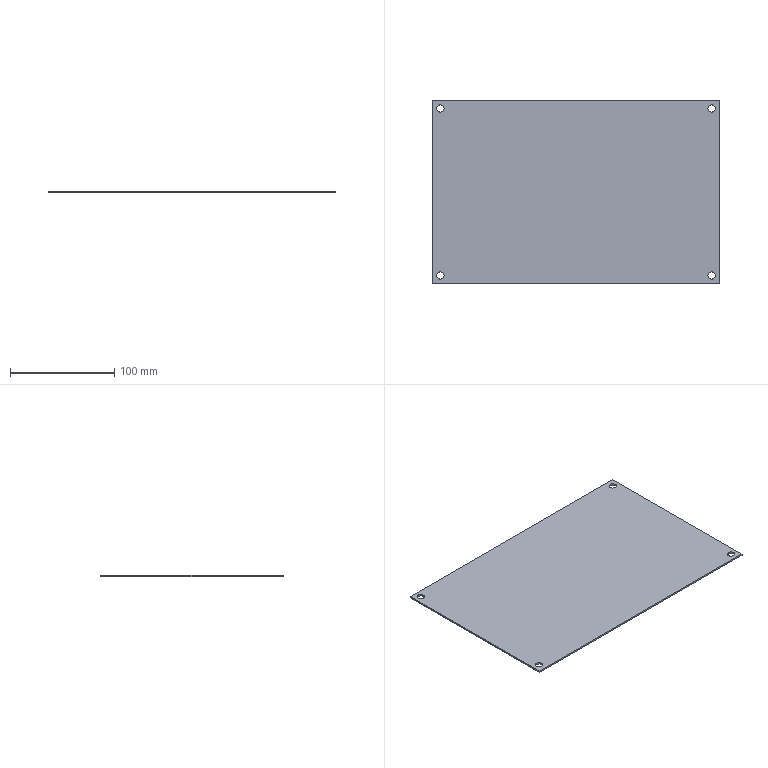Part | SolidWorks | features FlatPattern 1, ICE 1, SMBaseFlange 1, SheetMetal 1 | 1 solid | 14 faces | box 275 x 175 x 1.5 mm | volume 71957 mm3 | cylinder 8 | plane 6 | commonest cylinder face diameters 7 x8
STEP:
#1=CARTESIAN_POINT('',(-133.5,80.,-1.5));
#2=VERTEX_POINT('',#1);
#3=CARTESIAN_POINT('',(-126.5,80.,-1.5));
#4=VERTEX_POINT('',#3);
#5=CARTESIAN_POINT('',(-130.,80.,-1.5));
#6=DIRECTION('',(0.,0.,1.));
#7=DIRECTION('',(1.,0.,0.));
#8=AXIS2_PLACEMENT_3D('',#5,#6,#7);
#9=CIRCLE('',#8,3.5);
#10=EDGE_CURVE('',#2,#4,#9,.T.);
#11=ORIENTED_EDGE('',*,*,#10,.F.);
#12=CARTESIAN_POINT('',(-133.5,80.,0.));
#13=VERTEX_POINT('',#12);
#14=CARTESIAN_POINT('',(-133.5,80.,-10.));
#15=DIRECTION('',(0.,0.,1.));
#16=VECTOR('',#15,1000.);
#17=LINE('',#14,#16);
#18=EDGE_CURVE('',#2,#13,#17,.T.);
#19=ORIENTED_EDGE('',*,*,#18,.T.);
#20=CARTESIAN_POINT('',(-126.5,80.,0.));
#21=VERTEX_POINT('',#20);
#22=CARTESIAN_POINT('',(-130.,80.,0.));
#23=DIRECTION('',(0.,0.,1.));
#24=DIRECTION('',(-1.,0.,0.));
#25=AXIS2_PLACEMENT_3D('',#22,#23,#24);
#26=CIRCLE('',#25,3.5);
#27=EDGE_CURVE('',#13,#21,#26,.T.);
#28=ORIENTED_EDGE('',*,*,#27,.T.);
#29=CARTESIAN_POINT('',(-126.5,80.,-10.));
#30=DIRECTION('',(0.,0.,1.));
#31=VECTOR('',#30,1000.);
#32=LINE('',#29,#31);
#33=EDGE_CURVE('',#4,#21,#32,.T.);
#34=ORIENTED_EDGE('',*,*,#33,.F.);
#35=EDGE_LOOP('',(#11,#19,#28,#34));
#36=FACE_OUTER_BOUND('',#35,.T.);
#37=CARTESIAN_POINT('',(-130.,80.,-10.));
#38=DIRECTION('',(0.,0.,1.));
#39=DIRECTION('',(1.,0.,0.));
#40=AXIS2_PLACEMENT_3D('',#37,#38,#39);
#41=CYLINDRICAL_SURFACE('',#40,3.5);
#42=ADVANCED_FACE('',(#36),#41,.F.);
#43=CARTESIAN_POINT('',(-133.5,-80.,-1.5));
#44=VERTEX_POINT('',#43);
#45=CARTESIAN_POINT('',(-126.5,-80.,-1.5));
#46=VERTEX_POINT('',#45);
#47=CARTESIAN_POINT('',(-130.,-80.,-1.5));
#48=DIRECTION('',(0.,0.,1.));
#49=DIRECTION('',(1.,0.,0.));
#50=AXIS2_PLACEMENT_3D('',#47,#48,#49);
#51=CIRCLE('',#50,3.5);
#52=EDGE_CURVE('',#44,#46,#51,.T.);
#53=ORIENTED_EDGE('',*,*,#52,.F.);
#54=CARTESIAN_POINT('',(-133.5,-80.,0.));
#55=VERTEX_POINT('',#54);
#56=CARTESIAN_POINT('',(-133.5,-80.,-10.));
#57=DIRECTION('',(0.,0.,1.));
#58=VECTOR('',#57,1000.);
#59=LINE('',#56,#58);
#60=EDGE_CURVE('',#44,#55,#59,.T.);
#61=ORIENTED_EDGE('',*,*,#60,.T.);
#62=CARTESIAN_POINT('',(-126.5,-80.,0.));
#63=VERTEX_POINT('',#62);
#64=CARTESIAN_POINT('',(-130.,-80.,0.));
#65=DIRECTION('',(0.,0.,1.));
#66=DIRECTION('',(1.,0.,0.));
#67=AXIS2_PLACEMENT_3D('',#64,#65,#66);
#68=CIRCLE('',#67,3.5);
#69=EDGE_CURVE('',#55,#63,#68,.T.);
#70=ORIENTED_EDGE('',*,*,#69,.T.);
#71=CARTESIAN_POINT('',(-126.5,-80.,-10.));
#72=DIRECTION('',(0.,0.,1.));
#73=VECTOR('',#72,1000.);
#74=LINE('',#71,#73);
#75=EDGE_CURVE('',#46,#63,#74,.T.);
#76=ORIENTED_EDGE('',*,*,#75,.F.);
#77=EDGE_LOOP('',(#53,#61,#70,#76));
#78=FACE_OUTER_BOUND('',#77,.T.);
#79=CARTESIAN_POINT('',(-130.,-80.,-10.));
#80=DIRECTION('',(0.,0.,1.));
#81=DIRECTION('',(1.,0.,0.));
#82=AXIS2_PLACEMENT_3D('',#79,#80,#81);
#83=CYLINDRICAL_SURFACE('',#82,3.5);
#84=ADVANCED_FACE('',(#78),#83,.F.);
#85=CARTESIAN_POINT('',(126.5,-80.,-1.5));
#86=VERTEX_POINT('',#85);
#87=CARTESIAN_POINT('',(133.5,-80.,-1.5));
#88=VERTEX_POINT('',#87);
#89=CARTESIAN_POINT('',(130.,-80.,-1.5));
#90=DIRECTION('',(0.,0.,1.));
#91=DIRECTION('',(1.,0.,0.));
#92=AXIS2_PLACEMENT_3D('',#89,#90,#91);
#93=CIRCLE('',#92,3.5);
#94=EDGE_CURVE('',#86,#88,#93,.T.);
#95=ORIENTED_EDGE('',*,*,#94,.F.);
#96=CARTESIAN_POINT('',(126.5,-80.,0.));
#97=VERTEX_POINT('',#96);
#98=CARTESIAN_POINT('',(126.5,-80.,-10.));
#99=DIRECTION('',(0.,0.,1.));
#100=VECTOR('',#99,1000.);
#101=LINE('',#98,#100);
#102=EDGE_CURVE('',#86,#97,#101,.T.);
#103=ORIENTED_EDGE('',*,*,#102,.T.);
#104=CARTESIAN_POINT('',(133.5,-80.,0.));
#105=VERTEX_POINT('',#104);
#106=CARTESIAN_POINT('',(130.,-80.,0.));
#107=DIRECTION('',(0.,0.,1.));
#108=DIRECTION('',(-1.,0.,0.));
#109=AXIS2_PLACEMENT_3D('',#106,#107,#108);
#110=CIRCLE('',#109,3.5);
#111=EDGE_CURVE('',#97,#105,#110,.T.);
#112=ORIENTED_EDGE('',*,*,#111,.T.);
#113=CARTESIAN_POINT('',(133.5,-80.,-10.));
#114=DIRECTION('',(0.,0.,1.));
#115=VECTOR('',#114,1000.);
#116=LINE('',#113,#115);
#117=EDGE_CURVE('',#88,#105,#116,.T.);
#118=ORIENTED_EDGE('',*,*,#117,.F.);
#119=EDGE_LOOP('',(#95,#103,#112,#118));
#120=FACE_OUTER_BOUND('',#119,.T.);
#121=CARTESIAN_POINT('',(130.,-80.,-10.));
#122=DIRECTION('',(0.,0.,1.));
#123=DIRECTION('',(1.,0.,0.));
#124=AXIS2_PLACEMENT_3D('',#121,#122,#123);
#125=CYLINDRICAL_SURFACE('',#124,3.5);
#126=ADVANCED_FACE('',(#120),#125,.F.);
#127=CARTESIAN_POINT('',(126.5,80.,-1.5));
#128=VERTEX_POINT('',#127);
#129=CARTESIAN_POINT('',(133.5,80.,-1.5));
#130=VERTEX_POINT('',#129);
#131=CARTESIAN_POINT('',(130.,80.,-1.5));
#132=DIRECTION('',(0.,0.,1.));
#133=DIRECTION('',(1.,0.,0.));
#134=AXIS2_PLACEMENT_3D('',#131,#132,#133);
#135=CIRCLE('',#134,3.5);
#136=EDGE_CURVE('',#128,#130,#135,.T.);
#137=ORIENTED_EDGE('',*,*,#136,.F.);
#138=CARTESIAN_POINT('',(126.5,80.,0.));
#139=VERTEX_POINT('',#138);
#140=CARTESIAN_POINT('',(126.5,80.,-10.));
#141=DIRECTION('',(0.,0.,1.));
#142=VECTOR('',#141,1000.);
#143=LINE('',#140,#142);
#144=EDGE_CURVE('',#128,#139,#143,.T.);
#145=ORIENTED_EDGE('',*,*,#144,.T.);
#146=CARTESIAN_POINT('',(133.5,80.,0.));
#147=VERTEX_POINT('',#146);
#148=CARTESIAN_POINT('',(130.,80.,0.));
#149=DIRECTION('',(0.,0.,1.));
#150=DIRECTION('',(1.,0.,0.));
#151=AXIS2_PLACEMENT_3D('',#148,#149,#150);
#152=CIRCLE('',#151,3.5);
#153=EDGE_CURVE('',#139,#147,#152,.T.);
#154=ORIENTED_EDGE('',*,*,#153,.T.);
#155=CARTESIAN_POINT('',(133.5,80.,-10.));
#156=DIRECTION('',(0.,0.,1.));
#157=VECTOR('',#156,1000.);
#158=LINE('',#155,#157);
#159=EDGE_CURVE('',#130,#147,#158,.T.);
#160=ORIENTED_EDGE('',*,*,#159,.F.);
#161=EDGE_LOOP('',(#137,#145,#154,#160));
#162=FACE_OUTER_BOUND('',#161,.T.);
#163=CARTESIAN_POINT('',(130.,80.,-10.));
#164=DIRECTION('',(0.,0.,1.));
#165=DIRECTION('',(1.,0.,0.));
#166=AXIS2_PLACEMENT_3D('',#163,#164,#165);
#167=CYLINDRICAL_SURFACE('',#166,3.5);
#168=ADVANCED_FACE('',(#162),#167,.F.);
#169=CARTESIAN_POINT('',(137.5,-87.5,0.));
#170=VERTEX_POINT('',#169);
#171=CARTESIAN_POINT('',(137.5,87.5,0.));
#172=VERTEX_POINT('',#171);
#173=CARTESIAN_POINT('',(137.5,87.5,0.));
#174=DIRECTION('',(0.,1.,0.));
#175=VECTOR('',#174,1000.);
#176=LINE('',#173,#175);
#177=EDGE_CURVE('',#170,#172,#176,.T.);
#178=ORIENTED_EDGE('',*,*,#177,.F.);
#179=CARTESIAN_POINT('',(137.5,-87.5,-1.5));
#180=VERTEX_POINT('',#179);
#181=CARTESIAN_POINT('',(137.5,-87.5,-1.5));
#182=DIRECTION('',(0.,0.,1.));
#183=VECTOR('',#182,1000.);
#184=LINE('',#181,#183);
#185=EDGE_CURVE('',#180,#170,#184,.T.);
#186=ORIENTED_EDGE('',*,*,#185,.F.);
#187=CARTESIAN_POINT('',(137.5,87.5,-1.5));
#188=VERTEX_POINT('',#187);
#189=CARTESIAN_POINT('',(137.5,87.5,-1.5));
#190=DIRECTION('',(0.,1.,0.));
#191=VECTOR('',#190,1000.);
#192=LINE('',#189,#191);
#193=EDGE_CURVE('',#180,#188,#192,.T.);
#194=ORIENTED_EDGE('',*,*,#193,.T.);
#195=CARTESIAN_POINT('',(137.5,87.5,-1.5));
#196=DIRECTION('',(0.,0.,1.));
#197=VECTOR('',#196,1000.);
#198=LINE('',#195,#197);
#199=EDGE_CURVE('',#188,#172,#198,.T.);
#200=ORIENTED_EDGE('',*,*,#199,.T.);
#201=EDGE_LOOP('',(#178,#186,#194,#200));
#202=FACE_OUTER_BOUND('',#201,.T.);
#203=CARTESIAN_POINT('',(137.5,87.5,-1.5));
#204=DIRECTION('',(1.,0.,0.));
#205=DIRECTION('',(0.,0.,-1.));
#206=AXIS2_PLACEMENT_3D('',#203,#204,#205);
#207=PLANE('',#206);
#208=ADVANCED_FACE('',(#202),#207,.T.);
#209=CARTESIAN_POINT('',(-137.5,-87.5,0.));
#210=VERTEX_POINT('',#209);
#211=CARTESIAN_POINT('',(-137.5,-87.5,0.));
#212=DIRECTION('',(1.,0.,0.));
#213=VECTOR('',#212,1000.);
#214=LINE('',#211,#213);
#215=EDGE_CURVE('',#210,#170,#214,.T.);
#216=ORIENTED_EDGE('',*,*,#215,.F.);
#217=CARTESIAN_POINT('',(-137.5,-87.5,-1.5));
#218=VERTEX_POINT('',#217);
#219=CARTESIAN_POINT('',(-137.5,-87.5,-1.5));
#220=DIRECTION('',(0.,0.,1.));
#221=VECTOR('',#220,1000.);
#222=LINE('',#219,#221);
#223=EDGE_CURVE('',#218,#210,#222,.T.);
#224=ORIENTED_EDGE('',*,*,#223,.F.);
#225=CARTESIAN_POINT('',(-137.5,-87.5,-1.5));
#226=DIRECTION('',(1.,0.,0.));
#227=VECTOR('',#226,1000.);
#228=LINE('',#225,#227);
#229=EDGE_CURVE('',#218,#180,#228,.T.);
#230=ORIENTED_EDGE('',*,*,#229,.T.);
#231=ORIENTED_EDGE('',*,*,#185,.T.);
#232=EDGE_LOOP('',(#216,#224,#230,#231));
#233=FACE_OUTER_BOUND('',#232,.T.);
#234=CARTESIAN_POINT('',(-137.5,-87.5,-1.5));
#235=DIRECTION('',(0.,-1.,0.));
#236=DIRECTION('',(0.,0.,-1.));
#237=AXIS2_PLACEMENT_3D('',#234,#235,#236);
#238=PLANE('',#237);
#239=ADVANCED_FACE('',(#233),#238,.T.);
#240=CARTESIAN_POINT('',(-137.5,87.5,0.));
#241=VERTEX_POINT('',#240);
#242=CARTESIAN_POINT('',(-137.5,87.5,0.));
#243=DIRECTION('',(0.,-1.,0.));
#244=VECTOR('',#243,1000.);
#245=LINE('',#242,#244);
#246=EDGE_CURVE('',#241,#210,#245,.T.);
#247=ORIENTED_EDGE('',*,*,#246,.F.);
#248=CARTESIAN_POINT('',(-137.5,87.5,-1.5));
#249=VERTEX_POINT('',#248);
#250=CARTESIAN_POINT('',(-137.5,87.5,-1.5));
#251=DIRECTION('',(0.,0.,1.));
#252=VECTOR('',#251,1000.);
#253=LINE('',#250,#252);
#254=EDGE_CURVE('',#249,#241,#253,.T.);
#255=ORIENTED_EDGE('',*,*,#254,.F.);
#256=CARTESIAN_POINT('',(-137.5,87.5,-1.5));
#257=DIRECTION('',(0.,-1.,0.));
#258=VECTOR('',#257,1000.);
#259=LINE('',#256,#258);
#260=EDGE_CURVE('',#249,#218,#259,.T.);
#261=ORIENTED_EDGE('',*,*,#260,.T.);
#262=ORIENTED_EDGE('',*,*,#223,.T.);
#263=EDGE_LOOP('',(#247,#255,#261,#262));
#264=FACE_OUTER_BOUND('',#263,.T.);
#265=CARTESIAN_POINT('',(-137.5,87.5,-1.5));
#266=DIRECTION('',(-1.,0.,0.));
#267=DIRECTION('',(0.,-1.,0.));
#268=AXIS2_PLACEMENT_3D('',#265,#266,#267);
#269=PLANE('',#268);
#270=ADVANCED_FACE('',(#264),#269,.T.);
#271=CARTESIAN_POINT('',(-137.5,87.5,0.));
#272=DIRECTION('',(-1.,0.,0.));
#273=VECTOR('',#272,1000.);
#274=LINE('',#271,#273);
#275=EDGE_CURVE('',#172,#241,#274,.T.);
#276=ORIENTED_EDGE('',*,*,#275,.F.);
#277=ORIENTED_EDGE('',*,*,#199,.F.);
#278=CARTESIAN_POINT('',(-137.5,87.5,-1.5));
#279=DIRECTION('',(-1.,0.,0.));
#280=VECTOR('',#279,1000.);
#281=LINE('',#278,#280);
#282=EDGE_CURVE('',#188,#249,#281,.T.);
#283=ORIENTED_EDGE('',*,*,#282,.T.);
#284=ORIENTED_EDGE('',*,*,#254,.T.);
#285=EDGE_LOOP('',(#276,#277,#283,#284));
#286=FACE_OUTER_BOUND('',#285,.T.);
#287=CARTESIAN_POINT('',(-137.5,87.5,-1.5));
#288=DIRECTION('',(0.,1.,0.));
#289=DIRECTION('',(0.,0.,1.));
#290=AXIS2_PLACEMENT_3D('',#287,#288,#289);
#291=PLANE('',#290);
#292=ADVANCED_FACE('',(#286),#291,.T.);
#293=CARTESIAN_POINT('',(-130.,80.,-1.5));
#294=DIRECTION('',(0.,0.,1.));
#295=DIRECTION('',(1.,0.,0.));
#296=AXIS2_PLACEMENT_3D('',#293,#294,#295);
#297=CIRCLE('',#296,3.5);
#298=EDGE_CURVE('',#4,#2,#297,.T.);
#299=ORIENTED_EDGE('',*,*,#298,.T.);
#300=ORIENTED_EDGE('',*,*,#10,.T.);
#301=EDGE_LOOP('',(#299,#300));
#302=FACE_BOUND('',#301,.T.);
#303=CARTESIAN_POINT('',(-130.,-80.,-1.5));
#304=DIRECTION('',(0.,0.,1.));
#305=DIRECTION('',(1.,0.,0.));
#306=AXIS2_PLACEMENT_3D('',#303,#304,#305);
#307=CIRCLE('',#306,3.5);
#308=EDGE_CURVE('',#46,#44,#307,.T.);
#309=ORIENTED_EDGE('',*,*,#308,.T.);
#310=ORIENTED_EDGE('',*,*,#52,.T.);
#311=EDGE_LOOP('',(#309,#310));
#312=FACE_BOUND('',#311,.T.);
#313=CARTESIAN_POINT('',(130.,-80.,-1.5));
#314=DIRECTION('',(0.,0.,1.));
#315=DIRECTION('',(1.,0.,0.));
#316=AXIS2_PLACEMENT_3D('',#313,#314,#315);
#317=CIRCLE('',#316,3.5);
#318=EDGE_CURVE('',#88,#86,#317,.T.);
#319=ORIENTED_EDGE('',*,*,#318,.T.);
#320=ORIENTED_EDGE('',*,*,#94,.T.);
#321=EDGE_LOOP('',(#319,#320));
#322=FACE_BOUND('',#321,.T.);
#323=CARTESIAN_POINT('',(130.,80.,-1.5));
#324=DIRECTION('',(0.,0.,1.));
#325=DIRECTION('',(1.,0.,0.));
#326=AXIS2_PLACEMENT_3D('',#323,#324,#325);
#327=CIRCLE('',#326,3.5);
#328=EDGE_CURVE('',#130,#128,#327,.T.);
#329=ORIENTED_EDGE('',*,*,#328,.T.);
#330=ORIENTED_EDGE('',*,*,#136,.T.);
#331=EDGE_LOOP('',(#329,#330));
#332=FACE_BOUND('',#331,.T.);
#333=ORIENTED_EDGE('',*,*,#193,.F.);
#334=ORIENTED_EDGE('',*,*,#229,.F.);
#335=ORIENTED_EDGE('',*,*,#260,.F.);
#336=ORIENTED_EDGE('',*,*,#282,.F.);
#337=EDGE_LOOP('',(#333,#334,#335,#336));
#338=FACE_OUTER_BOUND('',#337,.T.);
#339=CARTESIAN_POINT('',(0.,0.,-1.5));
#340=DIRECTION('',(0.,0.,1.));
#341=DIRECTION('',(1.,0.,0.));
#342=AXIS2_PLACEMENT_3D('',#339,#340,#341);
#343=PLANE('',#342);
#344=ADVANCED_FACE('',(#302,#312,#322,#332,#338),#343,.F.);
#345=CARTESIAN_POINT('',(-130.,80.,0.));
#346=DIRECTION('',(0.,0.,1.));
#347=DIRECTION('',(-1.,0.,0.));
#348=AXIS2_PLACEMENT_3D('',#345,#346,#347);
#349=CIRCLE('',#348,3.5);
#350=EDGE_CURVE('',#21,#13,#349,.T.);
#351=ORIENTED_EDGE('',*,*,#350,.F.);
#352=ORIENTED_EDGE('',*,*,#27,.F.);
#353=EDGE_LOOP('',(#351,#352));
#354=FACE_BOUND('',#353,.T.);
#355=CARTESIAN_POINT('',(-130.,-80.,0.));
#356=DIRECTION('',(0.,0.,1.));
#357=DIRECTION('',(1.,0.,0.));
#358=AXIS2_PLACEMENT_3D('',#355,#356,#357);
#359=CIRCLE('',#358,3.5);
#360=EDGE_CURVE('',#63,#55,#359,.T.);
#361=ORIENTED_EDGE('',*,*,#360,.F.);
#362=ORIENTED_EDGE('',*,*,#69,.F.);
#363=EDGE_LOOP('',(#361,#362));
#364=FACE_BOUND('',#363,.T.);
#365=CARTESIAN_POINT('',(130.,-80.,0.));
#366=DIRECTION('',(0.,0.,1.));
#367=DIRECTION('',(-1.,0.,0.));
#368=AXIS2_PLACEMENT_3D('',#365,#366,#367);
#369=CIRCLE('',#368,3.5);
#370=EDGE_CURVE('',#105,#97,#369,.T.);
#371=ORIENTED_EDGE('',*,*,#370,.F.);
#372=ORIENTED_EDGE('',*,*,#111,.F.);
#373=EDGE_LOOP('',(#371,#372));
#374=FACE_BOUND('',#373,.T.);
#375=CARTESIAN_POINT('',(130.,80.,0.));
#376=DIRECTION('',(0.,0.,1.));
#377=DIRECTION('',(1.,0.,0.));
#378=AXIS2_PLACEMENT_3D('',#375,#376,#377);
#379=CIRCLE('',#378,3.5);
#380=EDGE_CURVE('',#147,#139,#379,.T.);
#381=ORIENTED_EDGE('',*,*,#380,.F.);
#382=ORIENTED_EDGE('',*,*,#153,.F.);
#383=EDGE_LOOP('',(#381,#382));
#384=FACE_BOUND('',#383,.T.);
#385=ORIENTED_EDGE('',*,*,#177,.T.);
#386=ORIENTED_EDGE('',*,*,#275,.T.);
#387=ORIENTED_EDGE('',*,*,#246,.T.);
#388=ORIENTED_EDGE('',*,*,#215,.T.);
#389=EDGE_LOOP('',(#385,#386,#387,#388));
#390=FACE_OUTER_BOUND('',#389,.T.);
#391=CARTESIAN_POINT('',(0.,0.,0.));
#392=DIRECTION('',(0.,0.,1.));
#393=DIRECTION('',(1.,0.,0.));
#394=AXIS2_PLACEMENT_3D('',#391,#392,#393);
#395=PLANE('',#394);
#396=ADVANCED_FACE('',(#354,#364,#374,#384,#390),#395,.T.);
#397=ORIENTED_EDGE('',*,*,#144,.F.);
#398=ORIENTED_EDGE('',*,*,#328,.F.);
#399=ORIENTED_EDGE('',*,*,#159,.T.);
#400=ORIENTED_EDGE('',*,*,#380,.T.);
#401=EDGE_LOOP('',(#397,#398,#399,#400));
#402=FACE_OUTER_BOUND('',#401,.T.);
#403=CARTESIAN_POINT('',(130.,80.,-10.));
#404=DIRECTION('',(0.,0.,1.));
#405=DIRECTION('',(1.,0.,0.));
#406=AXIS2_PLACEMENT_3D('',#403,#404,#405);
#407=CYLINDRICAL_SURFACE('',#406,3.5);
#408=ADVANCED_FACE('',(#402),#407,.F.);
#409=ORIENTED_EDGE('',*,*,#102,.F.);
#410=ORIENTED_EDGE('',*,*,#318,.F.);
#411=ORIENTED_EDGE('',*,*,#117,.T.);
#412=ORIENTED_EDGE('',*,*,#370,.T.);
#413=EDGE_LOOP('',(#409,#410,#411,#412));
#414=FACE_OUTER_BOUND('',#413,.T.);
#415=CARTESIAN_POINT('',(130.,-80.,-10.));
#416=DIRECTION('',(0.,0.,1.));
#417=DIRECTION('',(1.,0.,0.));
#418=AXIS2_PLACEMENT_3D('',#415,#416,#417);
#419=CYLINDRICAL_SURFACE('',#418,3.5);
#420=ADVANCED_FACE('',(#414),#419,.F.);
#421=ORIENTED_EDGE('',*,*,#60,.F.);
#422=ORIENTED_EDGE('',*,*,#308,.F.);
#423=ORIENTED_EDGE('',*,*,#75,.T.);
#424=ORIENTED_EDGE('',*,*,#360,.T.);
#425=EDGE_LOOP('',(#421,#422,#423,#424));
#426=FACE_OUTER_BOUND('',#425,.T.);
#427=CARTESIAN_POINT('',(-130.,-80.,-10.));
#428=DIRECTION('',(0.,0.,1.));
#429=DIRECTION('',(1.,0.,0.));
#430=AXIS2_PLACEMENT_3D('',#427,#428,#429);
#431=CYLINDRICAL_SURFACE('',#430,3.5);
#432=ADVANCED_FACE('',(#426),#431,.F.);
#433=ORIENTED_EDGE('',*,*,#18,.F.);
#434=ORIENTED_EDGE('',*,*,#298,.F.);
#435=ORIENTED_EDGE('',*,*,#33,.T.);
#436=ORIENTED_EDGE('',*,*,#350,.T.);
#437=EDGE_LOOP('',(#433,#434,#435,#436));
#438=FACE_OUTER_BOUND('',#437,.T.);
#439=CARTESIAN_POINT('',(-130.,80.,-10.));
#440=DIRECTION('',(0.,0.,1.));
#441=DIRECTION('',(1.,0.,0.));
#442=AXIS2_PLACEMENT_3D('',#439,#440,#441);
#443=CYLINDRICAL_SURFACE('',#442,3.5);
#444=ADVANCED_FACE('',(#438),#443,.F.);
#445=CLOSED_SHELL('',(#42,#84,#126,#168,#208,#239,#270,#292,#344,#396,#408,#420,#432,#444));
#446=MANIFOLD_SOLID_BREP('',#445);
#447=CARTESIAN_POINT('',(0.,0.,0.));
#448=DIRECTION('',(0.,0.,1.));
#449=DIRECTION('',(1.,0.,0.));
#450=AXIS2_PLACEMENT_3D('',#447,#448,#449);
#451=(LENGTH_UNIT()NAMED_UNIT(*)SI_UNIT(.MILLI.,.METRE.));
#452=UNCERTAINTY_MEASURE_WITH_UNIT(LENGTH_MEASURE(0.00001),#451,'','');
#453=(NAMED_UNIT(*)PLANE_ANGLE_UNIT()SI_UNIT($,.RADIAN.));
#454=(NAMED_UNIT(*)SI_UNIT($,.STERADIAN.)SOLID_ANGLE_UNIT());
#455=(GEOMETRIC_REPRESENTATION_CONTEXT(3)GLOBAL_UNCERTAINTY_ASSIGNED_CONTEXT((#452))GLOBAL_UNIT_ASSIGNED_CONTEXT((#451,#453,#454))REPRESENTATION_CONTEXT('',''));
#456=ADVANCED_BREP_SHAPE_REPRESENTATION('',(#446,#450),#455);